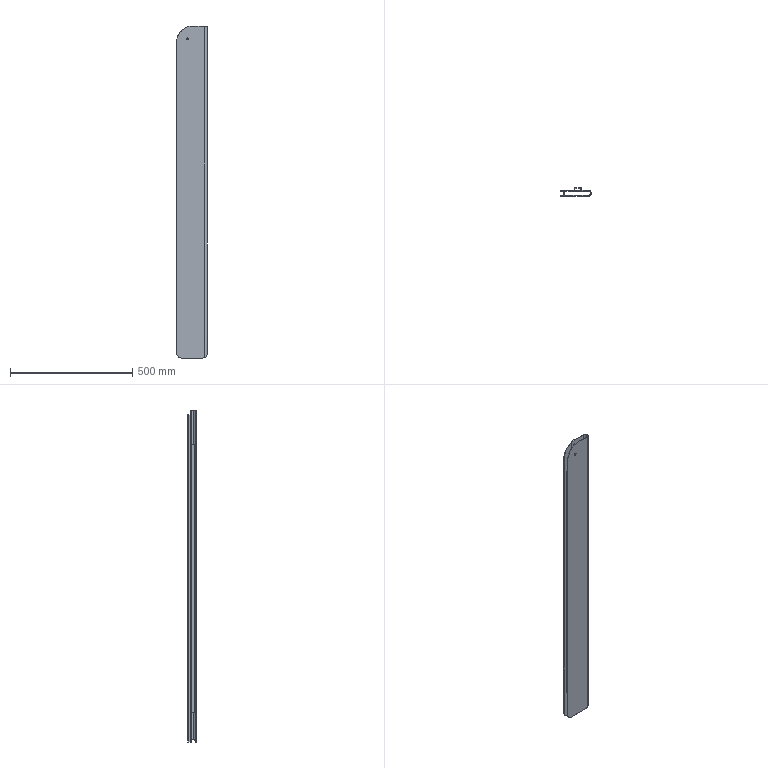Part | STEP file | 31E-01010TS12 | 1 solid | 73 faces | box 125 x 34 x 1360 mm | volume 828291 mm3 | cylinder 39 | plane 34 | commonest cylinder face diameters 1 x6 2 x6 0.6 x4 4 x4 40 x3 6 x2